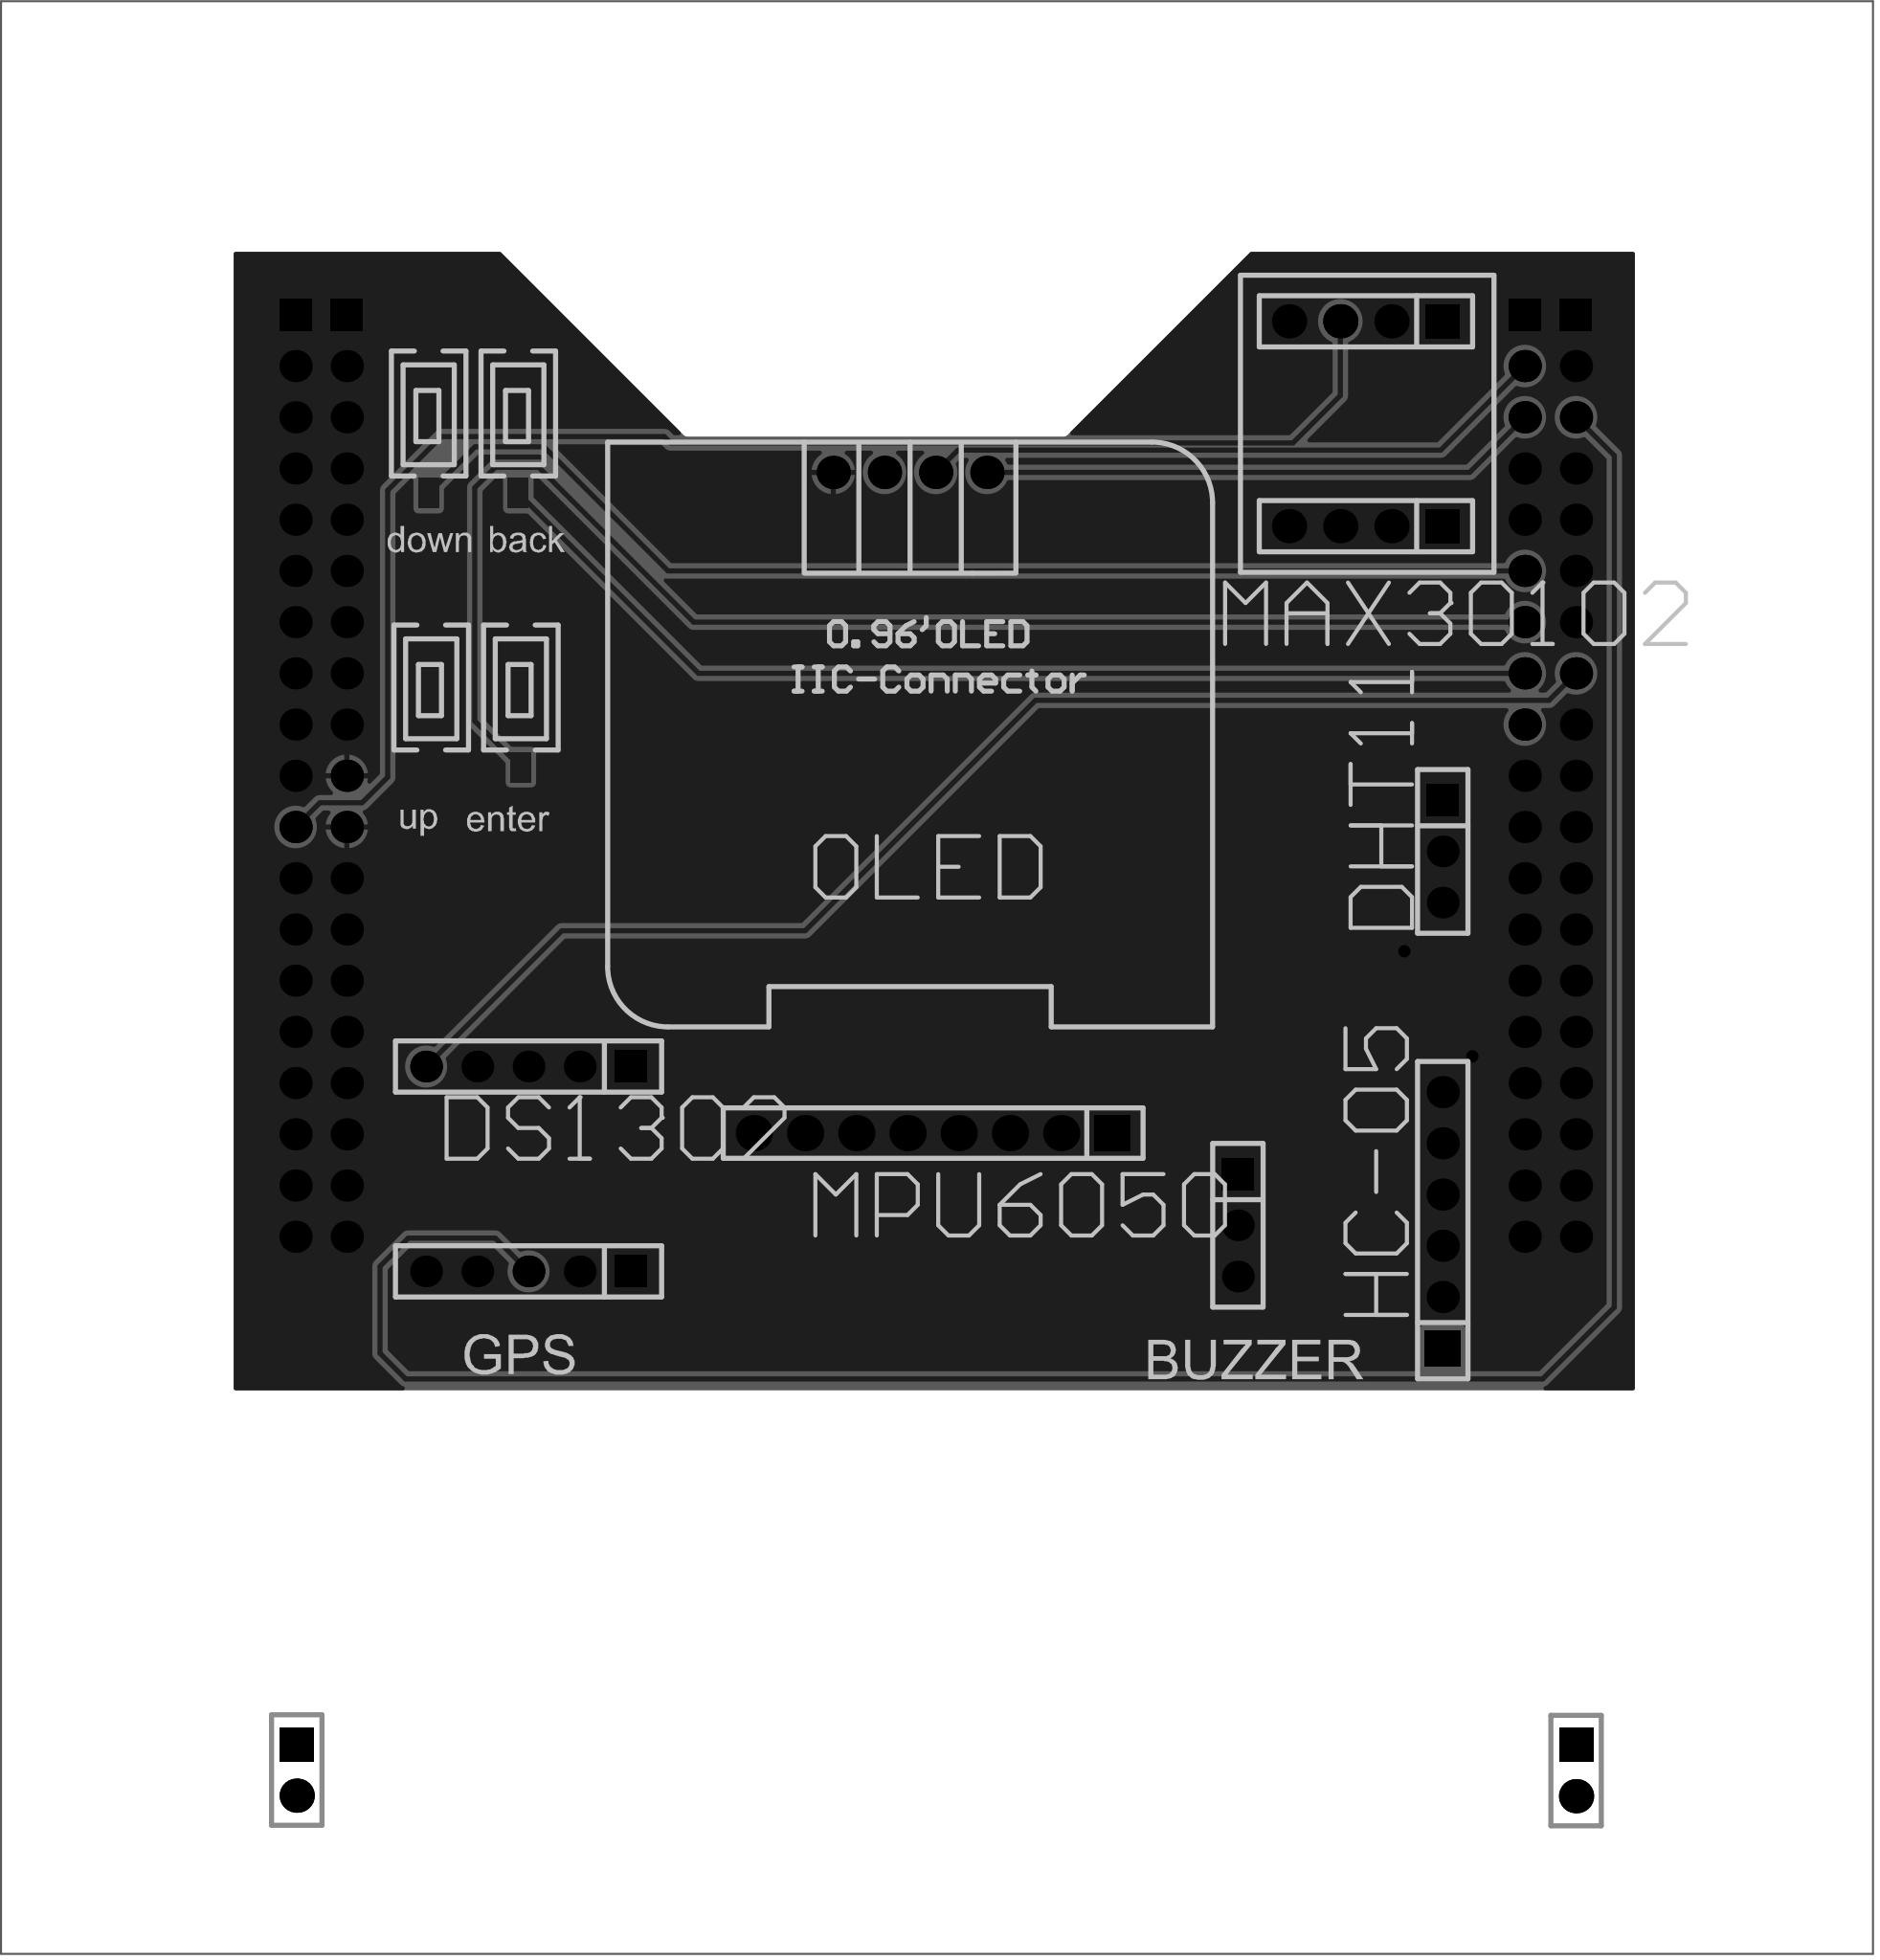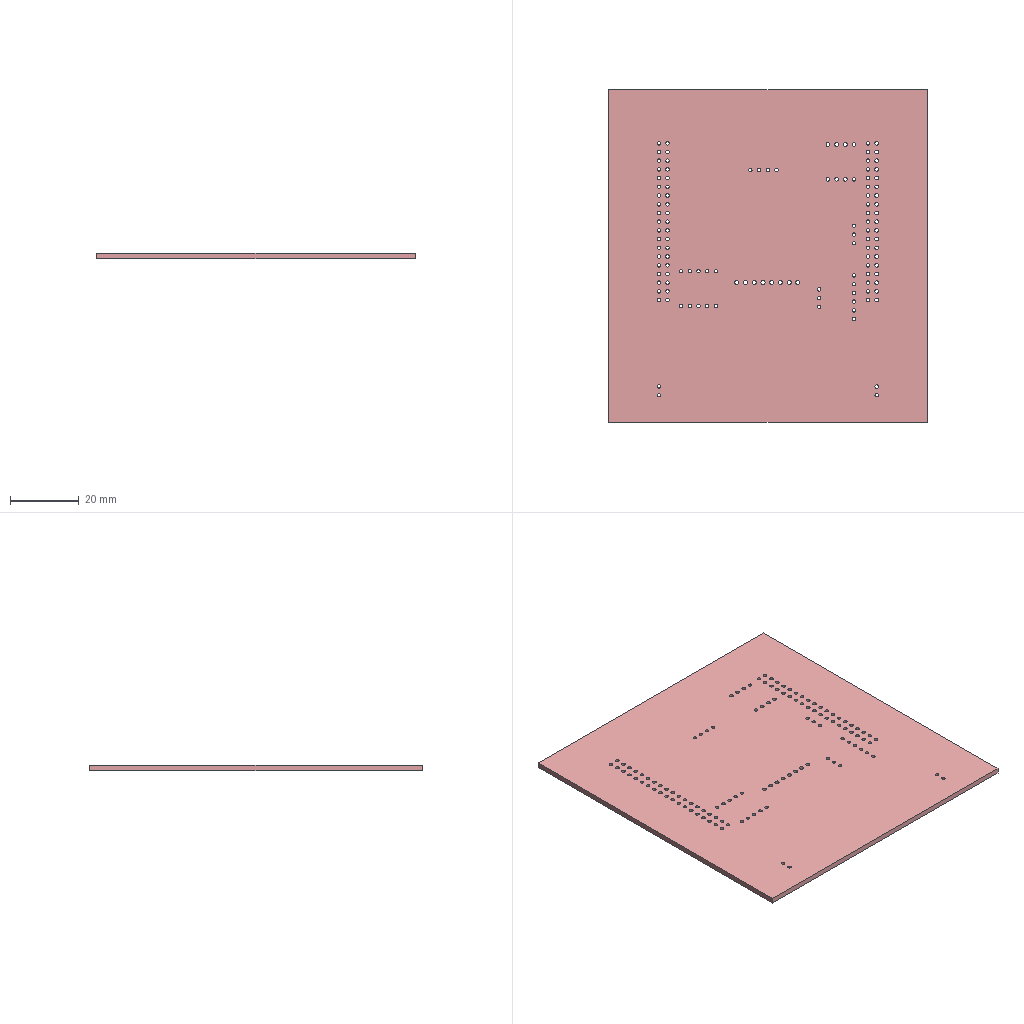Circuit board layout | Altium Designer | box 92.8 x 96.8 x 1.6 mm
Layer stack:
# Altium Designer layer stack of  (unit mm; dielectric type: 0 none, 1 core, 2 prepreg, 3 surface material)
index,name,kind,layer,copper_thickness_mm,dielectric_type,dielectric_thickness_mm,dielectric_material,dielectric_constant
0,Top Paste Mask Layer,other,,,,,,
1,Top Silkscreen Layer,other,,,,,,
2,Top Solder Mask Layer,dielectric,,,3,0.01,,3.3
3,Top Layer,copper,Top Layer,0.035,,,,
4,Dielectric1,dielectric,,,3,1.51,FR4,4.5
5,Bottom Layer,copper,Bottom Layer,0.035,,,,
6,Bottom Solder Mask Layer,dielectric,,,3,0.01,,3.3
7,Bottom Silkscreen Layer,other,,,,,,
8,Bottom Paste Mask Layer,other,,,,,,
# drill layer pairs: low layer,high layer
drill_pair,Top Layer,Bottom Layer
Part placement:
Designator,Comment,Layer,Footprint,Center-X(mm),Center-Y(mm),Rotation
H1,C2897382,BottomLayer,HDR-TH_19P-P2.54-V-F,84.459,128.276,270
H2,C2897382,BottomLayer,HDR-TH_19P-P2.54-V-F,86.999,128.276,270
H3,,TopLayer,HDR-TH_6P-P2.54-V-F,141.351,106.237,90
H4,,TopLayer,HDR-TH_8P-P2.54-V-F-1,116.078,110.555,180
H5,,TopLayer,HDR-TH_3P-P2.54-V-F,141.351,124.525,270
H6,,TopLayer,HDR-TH_3P-P2.54-V-F,131.191,105.983,270
H7,C2897382,BottomLayer,HDR-TH_19P-P2.54-V-F,145.419,128.276,270
H8,C2897382,BottomLayer,HDR-TH_19P-P2.54-V-F,147.959,128.276,270
H9,,TopLayer,HDR-TH_4P-P2.54-V-F,137.541,150.814,180
H10,,TopLayer,HDR-TH_4P-P2.54-V-F,137.541,140.654,180
H11,,TopLayer,HDR-TH_5P-P2.54-V-F,96.012,113.857,180
OLED1,,TopLayer,0.96OLED_4P,114.935,143.321,0
SW1,,TopLayer,Key_SMD_3.6x6.1x2.5,91.186,132.653,90
SW2,,TopLayer,Key_SMD_3.6x6.1x2.5,91.059,146.242,90
SW3,,TopLayer,Key_SMD_3.6x6.1x2.5,95.631,132.653,90
SW4,,TopLayer,Key_SMD_3.6x6.1x2.5,95.504,146.242,90
H12,,TopLayer,HDR-TH_5P-P2.54-V-F,96.012,103.697,180
H13,,BottomLayer,HDR-TH_2P-P2.54-V-F,84.517,78.967,270
H14,,BottomLayer,HDR-TH_2P-P2.54-V-F,147.963,78.94,270
Pad and via stacks:
# Altium Designer via and pad stacks of  (unit mm). Each distinct definition once, with the count of objects using it.
# via: kind,start_layer,end_layer,hole_mm,diameter_mm,mode(0 simple;1 top-mid-bottom;2 full stack),diameter_per_layer,count,example_net
# pad: kind,layer,hole_mm,hole_type(0 round;1 square;2 slot),plating,top_size,top_shape(1 round;2 rect;3 octagon;9 rounded rect),mid_size,bottom_size,mode,footprint,size_per_layer,count,example
pad,Multi-Layer,1.05,0,plated,1.6x1.6,1,1.6x1.6,1.6x1.6,0,HDR-TH_19P-P2.54-V-F,,72,H1.19
pad,Multi-Layer,1.05,0,plated,1.6x1.6,2,1.6x1.6,1.6x1.6,0,HDR-TH_19P-P2.54-V-F,,4,H1.1
pad,Multi-Layer,1.02,0,plated,1.6x1.6,1,1.6x1.6,1.6x1.6,0,HDR-TH_6P-P2.54-V-F,,5,H3.6
pad,Multi-Layer,1.02,0,plated,1.8x1.8,2,1.8x1.8,1.8x1.8,0,HDR-TH_6P-P2.54-V-F,,1,H3.1
pad,Multi-Layer,1.2,0,plated,1.8x1.8,2,1.8x1.8,1.8x1.8,0,HDR-TH_8P-P2.54-V-F-1,,1,H4.1
pad,Multi-Layer,1.2,0,plated,1.8x1.8,1,1.8x1.8,1.8x1.8,0,HDR-TH_8P-P2.54-V-F-1,,7,H4.2
pad,Multi-Layer,1.02,0,plated,1.575x1.575,1,1.575x1.575,1.575x1.575,0,HDR-TH_3P-P2.54-V-F,,4,H5.3
pad,Multi-Layer,1.02,0,plated,1.575x1.575,2,1.575x1.575,1.575x1.575,0,HDR-TH_3P-P2.54-V-F,,2,H5.1
pad,Multi-Layer,1.1,0,plated,1.7x1.7,2,1.7x1.7,1.7x1.7,0,HDR-TH_4P-P2.54-V-F,,2,H9.1
pad,Multi-Layer,1.1,0,plated,1.7x1.7,1,1.7x1.7,1.7x1.7,0,HDR-TH_4P-P2.54-V-F,,6,H9.2
pad,Multi-Layer,1.02,0,plated,1.575x1.575,1,1.575x1.575,1.575x1.575,0,HDR-TH_5P-P2.54-V-F,,8,H11.5
pad,Multi-Layer,1.02,0,plated,1.575x1.575,2,1.575x1.575,1.575x1.575,0,HDR-TH_5P-P2.54-V-F,,2,H11.1
pad,Multi-Layer,1,0,plated,1.65x1.65,1,1.65x1.65,1.65x1.65,0,0.96OLED_4P,,4,OLED1.4
pad,Multi-Layer,1,0,plated,1.7x1.7,2,1.7x1.7,1.7x1.7,0,HDR-TH_2P-P2.54-V-F,,2,H13.1
pad,Multi-Layer,1,0,plated,1.7x1.7,1,1.7x1.7,1.7x1.7,0,HDR-TH_2P-P2.54-V-F,,2,H13.2
pad,Top Layer,0,0,plated,1.501x1.001,2,1.501x1.001,1.501x1.001,0,Key_SMD_3.6x6.1x2.5,,8,SW1.2
via,Top Layer,Bottom Layer,0.3048,0.61,0,,2,CLK
Copper pours:
name,layer,net,type(0 solid;1 hatched;2 none)
Bottom Layer-GND,Bottom Layer,GND,0
Top Layer-GND,Top Layer,GND,0
Design rules, without the lines most boards share:
# Altium Designer design rules of  (exported by Altium Designer, unit mm)
# columns: name | kind | enabled | priority | scope1 | scope2 | descriptor | typed fields (field=value)
Copper_copperRegion_copperThickness1oz | 0 | disabled | 4 | All | All | Clearance Constraint (Gap=5.984mil) (Disabled)(All),(All) | gap=0.152
Copper_copperRegion_copperThickness1oz_1 | 63 | disabled | 4 | All | All | Board Clearance Constraint (Gap=0mil) (Disabled)(All) |
Copper_copperRegion_Copper_copperRegion | 0 | disabled | 5 | All | All | Clearance Constraint (Gap=5.984mil) (Disabled)(All),(All) | gap=0.152
Copper_copperRegion_Copper_copperRegion_1 | 63 | disabled | 5 | All | All | Board Clearance Constraint (Gap=0mil) (Disabled)(All) |
copperThickness1oz | 0 | enabled | 6 | All | All | Clearance Constraint (Gap=5.984mil) (All),(All) | gap=0.152
copperThickness1oz_1 | 63 | enabled | 6 | All | All | Board Clearance Constraint (Gap=0mil) (All) |
copperRegion_copperThickness1oz | 20 | disabled | 1 | All | All | Polygon Connect Rule(Relief Connect )(Conductor Width=10mil) (Relief Angle=90 Angle) (Entries=4) (Air Gap Width=10mil) (Disabled)(All),(All) | connect_style(0=relief,1=direct,2=none)=0 relief_conductor_width=0.254 relief_entries=4
copperRegion_Copper_copperRegion | 20 | disabled | 2 | All | All | Polygon Connect Rule(Relief Connect )(Conductor Width=10mil) (Relief Angle=90 Angle) (Entries=4) (Air Gap Width=10mil) (Disabled)(All),(All) | connect_style(0=relief,1=direct,2=none)=0 relief_conductor_width=0.254 relief_entries=4
copperRegion | 20 | enabled | 3 | All | All | Polygon Connect Rule(Relief Connect )(Conductor Width=10mil) (Relief Angle=90 Angle) (Entries=4) (Air Gap Width=10mil) (All),(All) | connect_style(0=relief,1=direct,2=none)=0 relief_conductor_width=0.254 relief_entries=4